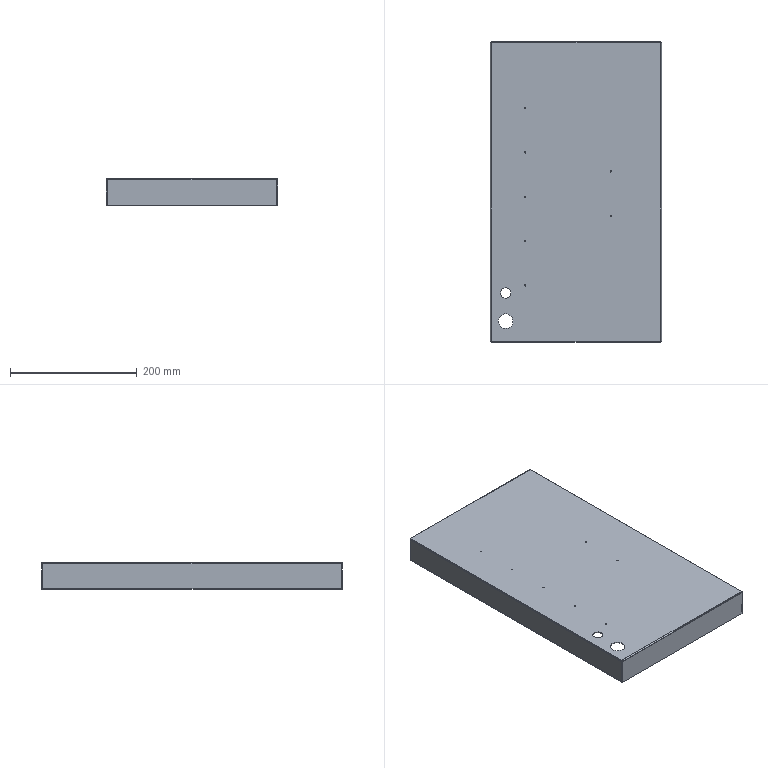Part | 1 solid | 66 faces | box 270 x 475 x 42 mm | volume 228367 mm3 | cylinder 30 | plane 28 | spline 8 | commonest cylinder face diameters 2 x14 1.473 x5 3.873 x5 16 x2 23 x2 25 x2